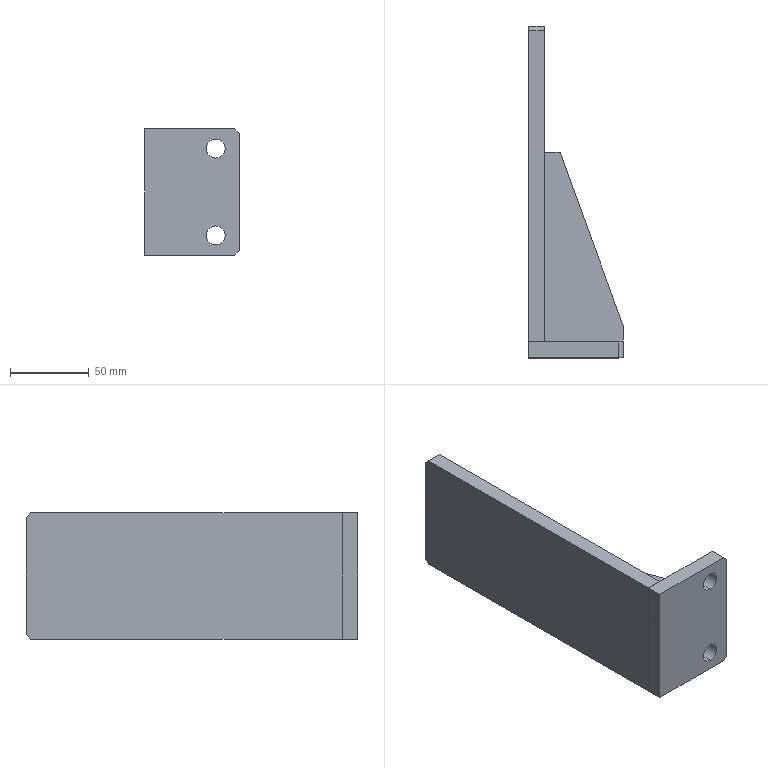Part | SolidWorks | features ICE 3, Chamfer 2, Extrusion 1 | 3 solids | 27 faces | box 60 x 210 x 80 mm | volume 235958 mm3 | plane 23 | cylinder 4 | commonest cylinder face diameters 12 x4
STEP:
#1=CARTESIAN_POINT('',(-30.,202.,40.));
#2=VERTEX_POINT('',#1);
#3=CARTESIAN_POINT('',(-30.,5.,40.));
#4=VERTEX_POINT('',#3);
#5=CARTESIAN_POINT('',(-30.,205.,40.));
#6=DIRECTION('',(0.,-1.,0.));
#7=VECTOR('',#6,1000.);
#8=LINE('',#5,#7);
#9=EDGE_CURVE('',#2,#4,#8,.T.);
#10=ORIENTED_EDGE('',*,*,#9,.F.);
#11=CARTESIAN_POINT('',(-30.,205.,37.));
#12=VERTEX_POINT('',#11);
#13=CARTESIAN_POINT('',(-30.,205.,37.));
#14=DIRECTION('',(0.,0.7071,-0.7071));
#15=VECTOR('',#14,1000.);
#16=LINE('',#13,#15);
#17=EDGE_CURVE('',#2,#12,#16,.T.);
#18=ORIENTED_EDGE('',*,*,#17,.T.);
#19=CARTESIAN_POINT('',(-30.,205.,-37.));
#20=VERTEX_POINT('',#19);
#21=CARTESIAN_POINT('',(-30.,205.,40.));
#22=DIRECTION('',(0.,0.,1.));
#23=VECTOR('',#22,1000.);
#24=LINE('',#21,#23);
#25=EDGE_CURVE('',#20,#12,#24,.T.);
#26=ORIENTED_EDGE('',*,*,#25,.F.);
#27=CARTESIAN_POINT('',(-30.,202.,-40.));
#28=VERTEX_POINT('',#27);
#29=CARTESIAN_POINT('',(-30.,205.,-37.));
#30=DIRECTION('',(0.,-0.7071,-0.7071));
#31=VECTOR('',#30,1000.);
#32=LINE('',#29,#31);
#33=EDGE_CURVE('',#20,#28,#32,.T.);
#34=ORIENTED_EDGE('',*,*,#33,.T.);
#35=CARTESIAN_POINT('',(-30.,5.,-40.));
#36=VERTEX_POINT('',#35);
#37=CARTESIAN_POINT('',(-30.,205.,-40.));
#38=DIRECTION('',(0.,-1.,0.));
#39=VECTOR('',#38,1000.);
#40=LINE('',#37,#39);
#41=EDGE_CURVE('',#28,#36,#40,.T.);
#42=ORIENTED_EDGE('',*,*,#41,.T.);
#43=CARTESIAN_POINT('',(-30.,5.,40.));
#44=DIRECTION('',(0.,0.,1.));
#45=VECTOR('',#44,1000.);
#46=LINE('',#43,#45);
#47=EDGE_CURVE('',#36,#4,#46,.T.);
#48=ORIENTED_EDGE('',*,*,#47,.T.);
#49=EDGE_LOOP('',(#10,#18,#26,#34,#42,#48));
#50=FACE_OUTER_BOUND('',#49,.T.);
#51=CARTESIAN_POINT('',(-30.,205.,40.));
#52=DIRECTION('',(1.,0.,0.));
#53=DIRECTION('',(0.,0.,-1.));
#54=AXIS2_PLACEMENT_3D('',#51,#52,#53);
#55=PLANE('',#54);
#56=ADVANCED_FACE('',(#50),#55,.F.);
#57=CARTESIAN_POINT('',(-20.,202.,40.));
#58=VERTEX_POINT('',#57);
#59=CARTESIAN_POINT('',(-20.,5.,40.));
#60=VERTEX_POINT('',#59);
#61=CARTESIAN_POINT('',(-20.,205.,40.));
#62=DIRECTION('',(0.,-1.,0.));
#63=VECTOR('',#62,1000.);
#64=LINE('',#61,#63);
#65=EDGE_CURVE('',#58,#60,#64,.T.);
#66=ORIENTED_EDGE('',*,*,#65,.F.);
#67=CARTESIAN_POINT('',(-30.,202.,40.));
#68=DIRECTION('',(-1.,0.,0.));
#69=VECTOR('',#68,1000.);
#70=LINE('',#67,#69);
#71=EDGE_CURVE('',#58,#2,#70,.T.);
#72=ORIENTED_EDGE('',*,*,#71,.T.);
#73=ORIENTED_EDGE('',*,*,#9,.T.);
#74=CARTESIAN_POINT('',(-30.,5.,40.));
#75=DIRECTION('',(1.,0.,0.));
#76=VECTOR('',#75,1000.);
#77=LINE('',#74,#76);
#78=EDGE_CURVE('',#4,#60,#77,.T.);
#79=ORIENTED_EDGE('',*,*,#78,.T.);
#80=EDGE_LOOP('',(#66,#72,#73,#79));
#81=FACE_OUTER_BOUND('',#80,.T.);
#82=CARTESIAN_POINT('',(-30.,205.,40.));
#83=DIRECTION('',(0.,0.,-1.));
#84=DIRECTION('',(-1.,0.,0.));
#85=AXIS2_PLACEMENT_3D('',#82,#83,#84);
#86=PLANE('',#85);
#87=ADVANCED_FACE('',(#81),#86,.F.);
#88=CARTESIAN_POINT('',(-20.,205.,37.));
#89=VERTEX_POINT('',#88);
#90=CARTESIAN_POINT('',(-20.,205.,-37.));
#91=VERTEX_POINT('',#90);
#92=CARTESIAN_POINT('',(-20.,205.,40.));
#93=DIRECTION('',(0.,0.,-1.));
#94=VECTOR('',#93,1000.);
#95=LINE('',#92,#94);
#96=EDGE_CURVE('',#89,#91,#95,.T.);
#97=ORIENTED_EDGE('',*,*,#96,.F.);
#98=CARTESIAN_POINT('',(-20.,205.,37.));
#99=DIRECTION('',(0.,-0.7071,0.7071));
#100=VECTOR('',#99,1000.);
#101=LINE('',#98,#100);
#102=EDGE_CURVE('',#89,#58,#101,.T.);
#103=ORIENTED_EDGE('',*,*,#102,.T.);
#104=ORIENTED_EDGE('',*,*,#65,.T.);
#105=CARTESIAN_POINT('',(-20.,5.,-40.));
#106=VERTEX_POINT('',#105);
#107=CARTESIAN_POINT('',(-20.,5.,40.));
#108=DIRECTION('',(0.,0.,-1.));
#109=VECTOR('',#108,1000.);
#110=LINE('',#107,#109);
#111=EDGE_CURVE('',#60,#106,#110,.T.);
#112=ORIENTED_EDGE('',*,*,#111,.T.);
#113=CARTESIAN_POINT('',(-20.,202.,-40.));
#114=VERTEX_POINT('',#113);
#115=CARTESIAN_POINT('',(-20.,205.,-40.));
#116=DIRECTION('',(0.,-1.,0.));
#117=VECTOR('',#116,1000.);
#118=LINE('',#115,#117);
#119=EDGE_CURVE('',#114,#106,#118,.T.);
#120=ORIENTED_EDGE('',*,*,#119,.F.);
#121=CARTESIAN_POINT('',(-20.,205.,-37.));
#122=DIRECTION('',(0.,0.7071,0.7071));
#123=VECTOR('',#122,1000.);
#124=LINE('',#121,#123);
#125=EDGE_CURVE('',#114,#91,#124,.T.);
#126=ORIENTED_EDGE('',*,*,#125,.T.);
#127=EDGE_LOOP('',(#97,#103,#104,#112,#120,#126));
#128=FACE_OUTER_BOUND('',#127,.T.);
#129=CARTESIAN_POINT('',(-20.,205.,40.));
#130=DIRECTION('',(-1.,0.,0.));
#131=DIRECTION('',(0.,0.,1.));
#132=AXIS2_PLACEMENT_3D('',#129,#130,#131);
#133=PLANE('',#132);
#134=ADVANCED_FACE('',(#128),#133,.F.);
#135=ORIENTED_EDGE('',*,*,#41,.F.);
#136=CARTESIAN_POINT('',(-30.,202.,-40.));
#137=DIRECTION('',(1.,0.,0.));
#138=VECTOR('',#137,1000.);
#139=LINE('',#136,#138);
#140=EDGE_CURVE('',#28,#114,#139,.T.);
#141=ORIENTED_EDGE('',*,*,#140,.T.);
#142=ORIENTED_EDGE('',*,*,#119,.T.);
#143=CARTESIAN_POINT('',(-30.,5.,-40.));
#144=DIRECTION('',(-1.,0.,0.));
#145=VECTOR('',#144,1000.);
#146=LINE('',#143,#145);
#147=EDGE_CURVE('',#106,#36,#146,.T.);
#148=ORIENTED_EDGE('',*,*,#147,.T.);
#149=EDGE_LOOP('',(#135,#141,#142,#148));
#150=FACE_OUTER_BOUND('',#149,.T.);
#151=CARTESIAN_POINT('',(-30.,205.,-40.));
#152=DIRECTION('',(0.,0.,1.));
#153=DIRECTION('',(1.,0.,0.));
#154=AXIS2_PLACEMENT_3D('',#151,#152,#153);
#155=PLANE('',#154);
#156=ADVANCED_FACE('',(#150),#155,.F.);
#157=ORIENTED_EDGE('',*,*,#25,.T.);
#158=CARTESIAN_POINT('',(0.,205.,37.));
#159=DIRECTION('',(1.,0.,0.));
#160=VECTOR('',#159,1000.);
#161=LINE('',#158,#160);
#162=EDGE_CURVE('',#12,#89,#161,.T.);
#163=ORIENTED_EDGE('',*,*,#162,.T.);
#164=ORIENTED_EDGE('',*,*,#96,.T.);
#165=CARTESIAN_POINT('',(0.,205.,-37.));
#166=DIRECTION('',(-1.,0.,0.));
#167=VECTOR('',#166,1000.);
#168=LINE('',#165,#167);
#169=EDGE_CURVE('',#91,#20,#168,.T.);
#170=ORIENTED_EDGE('',*,*,#169,.T.);
#171=EDGE_LOOP('',(#157,#163,#164,#170));
#172=FACE_OUTER_BOUND('',#171,.T.);
#173=CARTESIAN_POINT('',(0.,205.,0.));
#174=DIRECTION('',(0.,-1.,0.));
#175=DIRECTION('',(0.,0.,-1.));
#176=AXIS2_PLACEMENT_3D('',#173,#174,#175);
#177=PLANE('',#176);
#178=ADVANCED_FACE('',(#172),#177,.F.);
#179=ORIENTED_EDGE('',*,*,#47,.F.);
#180=ORIENTED_EDGE('',*,*,#147,.F.);
#181=ORIENTED_EDGE('',*,*,#111,.F.);
#182=ORIENTED_EDGE('',*,*,#78,.F.);
#183=EDGE_LOOP('',(#179,#180,#181,#182));
#184=FACE_OUTER_BOUND('',#183,.T.);
#185=CARTESIAN_POINT('',(0.,5.,0.));
#186=DIRECTION('',(0.,-1.,0.));
#187=DIRECTION('',(0.,0.,-1.));
#188=AXIS2_PLACEMENT_3D('',#185,#186,#187);
#189=PLANE('',#188);
#190=ADVANCED_FACE('',(#184),#189,.T.);
#191=ORIENTED_EDGE('',*,*,#17,.F.);
#192=ORIENTED_EDGE('',*,*,#71,.F.);
#193=ORIENTED_EDGE('',*,*,#102,.F.);
#194=ORIENTED_EDGE('',*,*,#162,.F.);
#195=EDGE_LOOP('',(#191,#192,#193,#194));
#196=FACE_OUTER_BOUND('',#195,.T.);
#197=CARTESIAN_POINT('',(0.,205.,37.));
#198=DIRECTION('',(0.,-0.7071,-0.7071));
#199=DIRECTION('',(1.,0.,0.));
#200=AXIS2_PLACEMENT_3D('',#197,#198,#199);
#201=PLANE('',#200);
#202=ADVANCED_FACE('',(#196),#201,.F.);
#203=ORIENTED_EDGE('',*,*,#125,.F.);
#204=ORIENTED_EDGE('',*,*,#140,.F.);
#205=ORIENTED_EDGE('',*,*,#33,.F.);
#206=ORIENTED_EDGE('',*,*,#169,.F.);
#207=EDGE_LOOP('',(#203,#204,#205,#206));
#208=FACE_OUTER_BOUND('',#207,.T.);
#209=CARTESIAN_POINT('',(0.,205.,-37.));
#210=DIRECTION('',(0.,-0.7071,0.7071));
#211=DIRECTION('',(-1.,0.,0.));
#212=AXIS2_PLACEMENT_3D('',#209,#210,#211);
#213=PLANE('',#212);
#214=ADVANCED_FACE('',(#208),#213,.F.);
#215=CLOSED_SHELL('',(#56,#87,#134,#156,#178,#190,#202,#214));
#216=MANIFOLD_SOLID_BREP('',#215);
#217=CARTESIAN_POINT('',(-20.,125.,-4.));
#218=VERTEX_POINT('',#217);
#219=CARTESIAN_POINT('',(-20.,5.,-4.));
#220=VERTEX_POINT('',#219);
#221=CARTESIAN_POINT('',(-20.,5.,-4.));
#222=DIRECTION('',(0.,-1.,0.));
#223=VECTOR('',#222,1000.);
#224=LINE('',#221,#223);
#225=EDGE_CURVE('',#218,#220,#224,.T.);
#226=ORIENTED_EDGE('',*,*,#225,.T.);
#227=CARTESIAN_POINT('',(-20.,5.,4.));
#228=VERTEX_POINT('',#227);
#229=CARTESIAN_POINT('',(-20.,5.,4.));
#230=DIRECTION('',(0.,0.,-1.));
#231=VECTOR('',#230,1000.);
#232=LINE('',#229,#231);
#233=EDGE_CURVE('',#228,#220,#232,.T.);
#234=ORIENTED_EDGE('',*,*,#233,.F.);
#235=CARTESIAN_POINT('',(-20.,125.,4.));
#236=VERTEX_POINT('',#235);
#237=CARTESIAN_POINT('',(-20.,5.,4.));
#238=DIRECTION('',(0.,-1.,0.));
#239=VECTOR('',#238,1000.);
#240=LINE('',#237,#239);
#241=EDGE_CURVE('',#236,#228,#240,.T.);
#242=ORIENTED_EDGE('',*,*,#241,.F.);
#243=CARTESIAN_POINT('',(-20.,125.,4.));
#244=DIRECTION('',(0.,0.,-1.));
#245=VECTOR('',#244,1000.);
#246=LINE('',#243,#245);
#247=EDGE_CURVE('',#236,#218,#246,.T.);
#248=ORIENTED_EDGE('',*,*,#247,.T.);
#249=EDGE_LOOP('',(#226,#234,#242,#248));
#250=FACE_OUTER_BOUND('',#249,.T.);
#251=CARTESIAN_POINT('',(-20.,5.,4.));
#252=DIRECTION('',(1.,0.,0.));
#253=DIRECTION('',(0.,0.,-1.));
#254=AXIS2_PLACEMENT_3D('',#251,#252,#253);
#255=PLANE('',#254);
#256=ADVANCED_FACE('',(#250),#255,.F.);
#257=CARTESIAN_POINT('',(30.,5.,-4.));
#258=VERTEX_POINT('',#257);
#259=CARTESIAN_POINT('',(30.,5.,-4.));
#260=DIRECTION('',(1.,0.,0.));
#261=VECTOR('',#260,1000.);
#262=LINE('',#259,#261);
#263=EDGE_CURVE('',#220,#258,#262,.T.);
#264=ORIENTED_EDGE('',*,*,#263,.T.);
#265=CARTESIAN_POINT('',(30.,5.,4.));
#266=VERTEX_POINT('',#265);
#267=CARTESIAN_POINT('',(30.,5.,4.));
#268=DIRECTION('',(0.,0.,-1.));
#269=VECTOR('',#268,1000.);
#270=LINE('',#267,#269);
#271=EDGE_CURVE('',#266,#258,#270,.T.);
#272=ORIENTED_EDGE('',*,*,#271,.F.);
#273=CARTESIAN_POINT('',(30.,5.,4.));
#274=DIRECTION('',(1.,0.,0.));
#275=VECTOR('',#274,1000.);
#276=LINE('',#273,#275);
#277=EDGE_CURVE('',#228,#266,#276,.T.);
#278=ORIENTED_EDGE('',*,*,#277,.F.);
#279=ORIENTED_EDGE('',*,*,#233,.T.);
#280=EDGE_LOOP('',(#264,#272,#278,#279));
#281=FACE_OUTER_BOUND('',#280,.T.);
#282=CARTESIAN_POINT('',(30.,5.,4.));
#283=DIRECTION('',(0.,1.,0.));
#284=DIRECTION('',(0.,0.,1.));
#285=AXIS2_PLACEMENT_3D('',#282,#283,#284);
#286=PLANE('',#285);
#287=ADVANCED_FACE('',(#281),#286,.F.);
#288=CARTESIAN_POINT('',(30.,15.,-4.));
#289=VERTEX_POINT('',#288);
#290=CARTESIAN_POINT('',(30.,15.,-4.));
#291=DIRECTION('',(0.,1.,0.));
#292=VECTOR('',#291,1000.);
#293=LINE('',#290,#292);
#294=EDGE_CURVE('',#258,#289,#293,.T.);
#295=ORIENTED_EDGE('',*,*,#294,.T.);
#296=CARTESIAN_POINT('',(30.,15.,4.));
#297=VERTEX_POINT('',#296);
#298=CARTESIAN_POINT('',(30.,15.,4.));
#299=DIRECTION('',(0.,0.,-1.));
#300=VECTOR('',#299,1000.);
#301=LINE('',#298,#300);
#302=EDGE_CURVE('',#297,#289,#301,.T.);
#303=ORIENTED_EDGE('',*,*,#302,.F.);
#304=CARTESIAN_POINT('',(30.,15.,4.));
#305=DIRECTION('',(0.,1.,0.));
#306=VECTOR('',#305,1000.);
#307=LINE('',#304,#306);
#308=EDGE_CURVE('',#266,#297,#307,.T.);
#309=ORIENTED_EDGE('',*,*,#308,.F.);
#310=ORIENTED_EDGE('',*,*,#271,.T.);
#311=EDGE_LOOP('',(#295,#303,#309,#310));
#312=FACE_OUTER_BOUND('',#311,.T.);
#313=CARTESIAN_POINT('',(30.,15.,4.));
#314=DIRECTION('',(-1.,0.,0.));
#315=DIRECTION('',(0.,0.,1.));
#316=AXIS2_PLACEMENT_3D('',#313,#314,#315);
#317=PLANE('',#316);
#318=ADVANCED_FACE('',(#312),#317,.F.);
#319=CARTESIAN_POINT('',(-10.,125.,-4.));
#320=VERTEX_POINT('',#319);
#321=CARTESIAN_POINT('',(-10.,125.,-4.));
#322=DIRECTION('',(-0.3417,0.9398,0.));
#323=VECTOR('',#322,1000.);
#324=LINE('',#321,#323);
#325=EDGE_CURVE('',#289,#320,#324,.T.);
#326=ORIENTED_EDGE('',*,*,#325,.T.);
#327=CARTESIAN_POINT('',(-10.,125.,4.));
#328=VERTEX_POINT('',#327);
#329=CARTESIAN_POINT('',(-10.,125.,4.));
#330=DIRECTION('',(0.,0.,-1.));
#331=VECTOR('',#330,1000.);
#332=LINE('',#329,#331);
#333=EDGE_CURVE('',#328,#320,#332,.T.);
#334=ORIENTED_EDGE('',*,*,#333,.F.);
#335=CARTESIAN_POINT('',(-10.,125.,4.));
#336=DIRECTION('',(-0.3417,0.9398,0.));
#337=VECTOR('',#336,1000.);
#338=LINE('',#335,#337);
#339=EDGE_CURVE('',#297,#328,#338,.T.);
#340=ORIENTED_EDGE('',*,*,#339,.F.);
#341=ORIENTED_EDGE('',*,*,#302,.T.);
#342=EDGE_LOOP('',(#326,#334,#340,#341));
#343=FACE_OUTER_BOUND('',#342,.T.);
#344=CARTESIAN_POINT('',(-10.,125.,4.));
#345=DIRECTION('',(-0.9398,-0.3417,0.));
#346=DIRECTION('',(0.3417,-0.9398,0.));
#347=AXIS2_PLACEMENT_3D('',#344,#345,#346);
#348=PLANE('',#347);
#349=ADVANCED_FACE('',(#343),#348,.F.);
#350=CARTESIAN_POINT('',(-20.,125.,-4.));
#351=DIRECTION('',(-1.,0.,0.));
#352=VECTOR('',#351,1000.);
#353=LINE('',#350,#352);
#354=EDGE_CURVE('',#320,#218,#353,.T.);
#355=ORIENTED_EDGE('',*,*,#354,.T.);
#356=ORIENTED_EDGE('',*,*,#247,.F.);
#357=CARTESIAN_POINT('',(-20.,125.,4.));
#358=DIRECTION('',(-1.,0.,0.));
#359=VECTOR('',#358,1000.);
#360=LINE('',#357,#359);
#361=EDGE_CURVE('',#328,#236,#360,.T.);
#362=ORIENTED_EDGE('',*,*,#361,.F.);
#363=ORIENTED_EDGE('',*,*,#333,.T.);
#364=EDGE_LOOP('',(#355,#356,#362,#363));
#365=FACE_OUTER_BOUND('',#364,.T.);
#366=CARTESIAN_POINT('',(-20.,125.,4.));
#367=DIRECTION('',(0.,-1.,0.));
#368=DIRECTION('',(0.,0.,-1.));
#369=AXIS2_PLACEMENT_3D('',#366,#367,#368);
#370=PLANE('',#369);
#371=ADVANCED_FACE('',(#365),#370,.F.);
#372=ORIENTED_EDGE('',*,*,#241,.T.);
#373=ORIENTED_EDGE('',*,*,#277,.T.);
#374=ORIENTED_EDGE('',*,*,#308,.T.);
#375=ORIENTED_EDGE('',*,*,#339,.T.);
#376=ORIENTED_EDGE('',*,*,#361,.T.);
#377=EDGE_LOOP('',(#372,#373,#374,#375,#376));
#378=FACE_OUTER_BOUND('',#377,.T.);
#379=CARTESIAN_POINT('',(0.,0.,4.));
#380=DIRECTION('',(0.,0.,-1.));
#381=DIRECTION('',(-1.,0.,0.));
#382=AXIS2_PLACEMENT_3D('',#379,#380,#381);
#383=PLANE('',#382);
#384=ADVANCED_FACE('',(#378),#383,.F.);
#385=ORIENTED_EDGE('',*,*,#225,.F.);
#386=ORIENTED_EDGE('',*,*,#354,.F.);
#387=ORIENTED_EDGE('',*,*,#325,.F.);
#388=ORIENTED_EDGE('',*,*,#294,.F.);
#389=ORIENTED_EDGE('',*,*,#263,.F.);
#390=EDGE_LOOP('',(#385,#386,#387,#388,#389));
#391=FACE_OUTER_BOUND('',#390,.T.);
#392=CARTESIAN_POINT('',(0.,0.,-4.));
#393=DIRECTION('',(0.,0.,-1.));
#394=DIRECTION('',(-1.,0.,0.));
#395=AXIS2_PLACEMENT_3D('',#392,#393,#394);
#396=PLANE('',#395);
#397=ADVANCED_FACE('',(#391),#396,.T.);
#398=CLOSED_SHELL('',(#256,#287,#318,#349,#371,#384,#397));
#399=MANIFOLD_SOLID_BREP('',#398);
#400=CARTESIAN_POINT('',(15.,-5.,21.5));
#401=VERTEX_POINT('',#400);
#402=CARTESIAN_POINT('',(15.,-5.,33.5));
#403=VERTEX_POINT('',#402);
#404=CARTESIAN_POINT('',(15.,-5.,27.5));
#405=DIRECTION('',(0.,1.,0.));
#406=DIRECTION('',(0.,0.,1.));
#407=AXIS2_PLACEMENT_3D('',#404,#405,#406);
#408=CIRCLE('',#407,6.);
#409=EDGE_CURVE('',#401,#403,#408,.T.);
#410=ORIENTED_EDGE('',*,*,#409,.F.);
#411=CARTESIAN_POINT('',(15.,5.,21.5));
#412=VERTEX_POINT('',#411);
#413=CARTESIAN_POINT('',(15.,-5.,21.5));
#414=DIRECTION('',(0.,1.,0.));
#415=VECTOR('',#414,1000.);
#416=LINE('',#413,#415);
#417=EDGE_CURVE('',#401,#412,#416,.T.);
#418=ORIENTED_EDGE('',*,*,#417,.T.);
#419=CARTESIAN_POINT('',(15.,5.,33.5));
#420=VERTEX_POINT('',#419);
#421=CARTESIAN_POINT('',(15.,5.,27.5));
#422=DIRECTION('',(0.,1.,0.));
#423=DIRECTION('',(0.,0.,1.));
#424=AXIS2_PLACEMENT_3D('',#421,#422,#423);
#425=CIRCLE('',#424,6.);
#426=EDGE_CURVE('',#412,#420,#425,.T.);
#427=ORIENTED_EDGE('',*,*,#426,.T.);
#428=CARTESIAN_POINT('',(15.,-5.,33.5));
#429=DIRECTION('',(0.,1.,0.));
#430=VECTOR('',#429,1000.);
#431=LINE('',#428,#430);
#432=EDGE_CURVE('',#403,#420,#431,.T.);
#433=ORIENTED_EDGE('',*,*,#432,.F.);
#434=EDGE_LOOP('',(#410,#418,#427,#433));
#435=FACE_OUTER_BOUND('',#434,.T.);
#436=CARTESIAN_POINT('',(15.,-5.,27.5));
#437=DIRECTION('',(0.,1.,0.));
#438=DIRECTION('',(0.,0.,1.));
#439=AXIS2_PLACEMENT_3D('',#436,#437,#438);
#440=CYLINDRICAL_SURFACE('',#439,6.);
#441=ADVANCED_FACE('',(#435),#440,.F.);
#442=CARTESIAN_POINT('',(15.,-5.,-33.5));
#443=VERTEX_POINT('',#442);
#444=CARTESIAN_POINT('',(15.,-5.,-21.5));
#445=VERTEX_POINT('',#444);
#446=CARTESIAN_POINT('',(15.,-5.,-27.5));
#447=DIRECTION('',(0.,1.,0.));
#448=DIRECTION('',(0.,0.,-1.));
#449=AXIS2_PLACEMENT_3D('',#446,#447,#448);
#450=CIRCLE('',#449,6.);
#451=EDGE_CURVE('',#443,#445,#450,.T.);
#452=ORIENTED_EDGE('',*,*,#451,.F.);
#453=CARTESIAN_POINT('',(15.,5.,-33.5));
#454=VERTEX_POINT('',#453);
#455=CARTESIAN_POINT('',(15.,-5.,-33.5));
#456=DIRECTION('',(0.,1.,0.));
#457=VECTOR('',#456,1000.);
#458=LINE('',#455,#457);
#459=EDGE_CURVE('',#443,#454,#458,.T.);
#460=ORIENTED_EDGE('',*,*,#459,.T.);
#461=CARTESIAN_POINT('',(15.,5.,-21.5));
#462=VERTEX_POINT('',#461);
#463=CARTESIAN_POINT('',(15.,5.,-27.5));
#464=DIRECTION('',(0.,1.,0.));
#465=DIRECTION('',(0.,0.,-1.));
#466=AXIS2_PLACEMENT_3D('',#463,#464,#465);
#467=CIRCLE('',#466,6.);
#468=EDGE_CURVE('',#454,#462,#467,.T.);
#469=ORIENTED_EDGE('',*,*,#468,.T.);
#470=CARTESIAN_POINT('',(15.,-5.,-21.5));
#471=DIRECTION('',(0.,1.,0.));
#472=VECTOR('',#471,1000.);
#473=LINE('',#470,#472);
#474=EDGE_CURVE('',#445,#462,#473,.T.);
#475=ORIENTED_EDGE('',*,*,#474,.F.);
#476=EDGE_LOOP('',(#452,#460,#469,#475));
#477=FACE_OUTER_BOUND('',#476,.T.);
#478=CARTESIAN_POINT('',(15.,-5.,-27.5));
#479=DIRECTION('',(0.,1.,0.));
#480=DIRECTION('',(0.,0.,1.));
#481=AXIS2_PLACEMENT_3D('',#478,#479,#480);
#482=CYLINDRICAL_SURFACE('',#481,6.);
#483=ADVANCED_FACE('',(#477),#482,.F.);
#484=CARTESIAN_POINT('',(30.,-5.,37.));
#485=VERTEX_POINT('',#484);
#486=CARTESIAN_POINT('',(30.,-5.,-37.));
#487=VERTEX_POINT('',#486);
#488=CARTESIAN_POINT('',(30.,-5.,40.));
#489=DIRECTION('',(0.,0.,-1.));
#490=VECTOR('',#489,1000.);
#491=LINE('',#488,#490);
#492=EDGE_CURVE('',#485,#487,#491,.T.);
#493=ORIENTED_EDGE('',*,*,#492,.T.);
#494=CARTESIAN_POINT('',(30.,5.,-37.));
#495=VERTEX_POINT('',#494);
#496=CARTESIAN_POINT('',(30.,5.,-37.));
#497=DIRECTION('',(0.,1.,0.));
#498=VECTOR('',#497,1000.);
#499=LINE('',#496,#498);
#500=EDGE_CURVE('',#487,#495,#499,.T.);
#501=ORIENTED_EDGE('',*,*,#500,.T.);
#502=CARTESIAN_POINT('',(30.,5.,37.));
#503=VERTEX_POINT('',#502);
#504=CARTESIAN_POINT('',(30.,5.,40.));
#505=DIRECTION('',(0.,0.,-1.));
#506=VECTOR('',#505,1000.);
#507=LINE('',#504,#506);
#508=EDGE_CURVE('',#503,#495,#507,.T.);
#509=ORIENTED_EDGE('',*,*,#508,.F.);
#510=CARTESIAN_POINT('',(30.,5.,37.));
#511=DIRECTION('',(0.,-1.,0.));
#512=VECTOR('',#511,1000.);
#513=LINE('',#510,#512);
#514=EDGE_CURVE('',#503,#485,#513,.T.);
#515=ORIENTED_EDGE('',*,*,#514,.T.);
#516=EDGE_LOOP('',(#493,#501,#509,#515));
#517=FACE_OUTER_BOUND('',#516,.T.);
#518=CARTESIAN_POINT('',(30.,5.,40.));
#519=DIRECTION('',(-1.,0.,0.));
#520=DIRECTION('',(0.,0.,1.));
#521=AXIS2_PLACEMENT_3D('',#518,#519,#520);
#522=PLANE('',#521);
#523=ADVANCED_FACE('',(#517),#522,.F.);
#524=CARTESIAN_POINT('',(27.,5.,-40.));
#525=VERTEX_POINT('',#524);
#526=CARTESIAN_POINT('',(-30.,5.,-40.));
#527=VERTEX_POINT('',#526);
#528=CARTESIAN_POINT('',(-30.,5.,-40.));
#529=DIRECTION('',(-1.,0.,0.));
#530=VECTOR('',#529,1000.);
#531=LINE('',#528,#530);
#532=EDGE_CURVE('',#525,#527,#531,.T.);
#533=ORIENTED_EDGE('',*,*,#532,.F.);
#534=CARTESIAN_POINT('',(27.,-5.,-40.));
#535=VERTEX_POINT('',#534);
#536=CARTESIAN_POINT('',(27.,5.,-40.));
#537=DIRECTION('',(0.,-1.,0.));
#538=VECTOR('',#537,1000.);
#539=LINE('',#536,#538);
#540=EDGE_CURVE('',#525,#535,#539,.T.);
#541=ORIENTED_EDGE('',*,*,#540,.T.);
#542=CARTESIAN_POINT('',(-30.,-5.,-40.));
#543=VERTEX_POINT('',#542);
#544=CARTESIAN_POINT('',(-30.,-5.,-40.));
#545=DIRECTION('',(-1.,0.,0.));
#546=VECTOR('',#545,1000.);
#547=LINE('',#544,#546);
#548=EDGE_CURVE('',#535,#543,#547,.T.);
#549=ORIENTED_EDGE('',*,*,#548,.T.);
#550=CARTESIAN_POINT('',(-30.,5.,-40.));
#551=DIRECTION('',(0.,-1.,0.));
#552=VECTOR('',#551,1000.);
#553=LINE('',#550,#552);
#554=EDGE_CURVE('',#527,#543,#553,.T.);
#555=ORIENTED_EDGE('',*,*,#554,.F.);
#556=EDGE_LOOP('',(#533,#541,#549,#555));
#557=FACE_OUTER_BOUND('',#556,.T.);
#558=CARTESIAN_POINT('',(-30.,5.,-40.));
#559=DIRECTION('',(0.,0.,1.));
#560=DIRECTION('',(1.,0.,0.));
#561=AXIS2_PLACEMENT_3D('',#558,#559,#560);
#562=PLANE('',#561);
#563=ADVANCED_FACE('',(#557),#562,.F.);
#564=CARTESIAN_POINT('',(-30.,-5.,40.));
#565=VERTEX_POINT('',#564);
#566=CARTESIAN_POINT('',(-30.,-5.,40.));
#567=DIRECTION('',(0.,0.,1.));
#568=VECTOR('',#567,1000.);
#569=LINE('',#566,#568);
#570=EDGE_CURVE('',#543,#565,#569,.T.);
#571=ORIENTED_EDGE('',*,*,#570,.T.);
#572=CARTESIAN_POINT('',(-30.,5.,40.));
#573=VERTEX_POINT('',#572);
#574=CARTESIAN_POINT('',(-30.,5.,40.));
#575=DIRECTION('',(0.,-1.,0.));
#576=VECTOR('',#575,1000.);
#577=LINE('',#574,#576);
#578=EDGE_CURVE('',#573,#565,#577,.T.);
#579=ORIENTED_EDGE('',*,*,#578,.F.);
#580=CARTESIAN_POINT('',(-30.,5.,40.));
#581=DIRECTION('',(0.,0.,1.));
#582=VECTOR('',#581,1000.);
#583=LINE('',#580,#582);
#584=EDGE_CURVE('',#527,#573,#583,.T.);
#585=ORIENTED_EDGE('',*,*,#584,.F.);
#586=ORIENTED_EDGE('',*,*,#554,.T.);
#587=EDGE_LOOP('',(#571,#579,#585,#586));
#588=FACE_OUTER_BOUND('',#587,.T.);
#589=CARTESIAN_POINT('',(-30.,5.,40.));
#590=DIRECTION('',(1.,0.,0.));
#591=DIRECTION('',(0.,0.,-1.));
#592=AXIS2_PLACEMENT_3D('',#589,#590,#591);
#593=PLANE('',#592);
#594=ADVANCED_FACE('',(#588),#593,.F.);
#595=CARTESIAN_POINT('',(27.,-5.,40.));
#596=VERTEX_POINT('',#595);
#597=CARTESIAN_POINT('',(-30.,-5.,40.));
#598=DIRECTION('',(1.,0.,0.));
#599=VECTOR('',#598,1000.);
#600=LINE('',#597,#599);
#601=EDGE_CURVE('',#565,#596,#600,.T.);
#602=ORIENTED_EDGE('',*,*,#601,.T.);
#603=CARTESIAN_POINT('',(27.,5.,40.));
#604=VERTEX_POINT('',#603);
#605=CARTESIAN_POINT('',(27.,5.,40.));
#606=DIRECTION('',(0.,1.,0.));
#607=VECTOR('',#606,1000.);
#608=LINE('',#605,#607);
#609=EDGE_CURVE('',#596,#604,#608,.T.);
#610=ORIENTED_EDGE('',*,*,#609,.T.);
#611=CARTESIAN_POINT('',(-30.,5.,40.));
#612=DIRECTION('',(1.,0.,0.));
#613=VECTOR('',#612,1000.);
#614=LINE('',#611,#613);
#615=EDGE_CURVE('',#573,#604,#614,.T.);
#616=ORIENTED_EDGE('',*,*,#615,.F.);
#617=ORIENTED_EDGE('',*,*,#578,.T.);
#618=EDGE_LOOP('',(#602,#610,#616,#617));
#619=FACE_OUTER_BOUND('',#618,.T.);
#620=CARTESIAN_POINT('',(-30.,5.,40.));
#621=DIRECTION('',(0.,0.,-1.));
#622=DIRECTION('',(-1.,0.,0.));
#623=AXIS2_PLACEMENT_3D('',#620,#621,#622);
#624=PLANE('',#623);
#625=ADVANCED_FACE('',(#619),#624,.F.);
#626=CARTESIAN_POINT('',(15.,5.,27.5));
#627=DIRECTION('',(0.,1.,0.));
#628=DIRECTION('',(0.,0.,1.));
#629=AXIS2_PLACEMENT_3D('',#626,#627,#628);
#630=CIRCLE('',#629,6.);
#631=EDGE_CURVE('',#420,#412,#630,.T.);
#632=ORIENTED_EDGE('',*,*,#631,.F.);
#633=ORIENTED_EDGE('',*,*,#426,.F.);
#634=EDGE_LOOP('',(#632,#633));
#635=FACE_BOUND('',#634,.T.);
#636=CARTESIAN_POINT('',(15.,5.,-27.5));
#637=DIRECTION('',(0.,1.,0.));
#638=DIRECTION('',(0.,0.,-1.));
#639=AXIS2_PLACEMENT_3D('',#636,#637,#638);
#640=CIRCLE('',#639,6.);
#641=EDGE_CURVE('',#462,#454,#640,.T.);
#642=ORIENTED_EDGE('',*,*,#641,.F.);
#643=ORIENTED_EDGE('',*,*,#468,.F.);
#644=EDGE_LOOP('',(#642,#643));
#645=FACE_BOUND('',#644,.T.);
#646=ORIENTED_EDGE('',*,*,#508,.T.);
#647=CARTESIAN_POINT('',(27.,5.,-40.));
#648=DIRECTION('',(-0.7071,0.,-0.7071));
#649=VECTOR('',#648,1000.);
#650=LINE('',#647,#649);
#651=EDGE_CURVE('',#495,#525,#650,.T.);
#652=ORIENTED_EDGE('',*,*,#651,.T.);
#653=ORIENTED_EDGE('',*,*,#532,.T.);
#654=ORIENTED_EDGE('',*,*,#584,.T.);
#655=ORIENTED_EDGE('',*,*,#615,.T.);
#656=CARTESIAN_POINT('',(30.,5.,37.));
#657=DIRECTION('',(0.7071,0.,-0.7071));
#658=VECTOR('',#657,1000.);
#659=LINE('',#656,#658);
#660=EDGE_CURVE('',#604,#503,#659,.T.);
#661=ORIENTED_EDGE('',*,*,#660,.T.);
#662=EDGE_LOOP('',(#646,#652,#653,#654,#655,#661));
#663=FACE_OUTER_BOUND('',#662,.T.);
#664=CARTESIAN_POINT('',(0.,5.,0.));
#665=DIRECTION('',(0.,-1.,0.));
#666=DIRECTION('',(0.,0.,-1.));
#667=AXIS2_PLACEMENT_3D('',#664,#665,#666);
#668=PLANE('',#667);
#669=ADVANCED_FACE('',(#635,#645,#663),#668,.F.);
#670=CARTESIAN_POINT('',(15.,-5.,27.5));
#671=DIRECTION('',(0.,1.,0.));
#672=DIRECTION('',(0.,0.,1.));
#673=AXIS2_PLACEMENT_3D('',#670,#671,#672);
#674=CIRCLE('',#673,6.);
#675=EDGE_CURVE('',#403,#401,#674,.T.);
#676=ORIENTED_EDGE('',*,*,#675,.T.);
#677=ORIENTED_EDGE('',*,*,#409,.T.);
#678=EDGE_LOOP('',(#676,#677));
#679=FACE_BOUND('',#678,.T.);
#680=CARTESIAN_POINT('',(15.,-5.,-27.5));
#681=DIRECTION('',(0.,1.,0.));
#682=DIRECTION('',(0.,0.,-1.));
#683=AXIS2_PLACEMENT_3D('',#680,#681,#682);
#684=CIRCLE('',#683,6.);
#685=EDGE_CURVE('',#445,#443,#684,.T.);
#686=ORIENTED_EDGE('',*,*,#685,.T.);
#687=ORIENTED_EDGE('',*,*,#451,.T.);
#688=EDGE_LOOP('',(#686,#687));
#689=FACE_BOUND('',#688,.T.);
#690=ORIENTED_EDGE('',*,*,#548,.F.);
#691=CARTESIAN_POINT('',(33.5,-5.,-33.5));
#692=DIRECTION('',(0.7071,0.,0.7071));
#693=VECTOR('',#692,1000.);
#694=LINE('',#691,#693);
#695=EDGE_CURVE('',#535,#487,#694,.T.);
#696=ORIENTED_EDGE('',*,*,#695,.T.);
#697=ORIENTED_EDGE('',*,*,#492,.F.);
#698=CARTESIAN_POINT('',(33.5,-5.,33.5));
#699=DIRECTION('',(-0.7071,0.,0.7071));
#700=VECTOR('',#699,1000.);
#701=LINE('',#698,#700);
#702=EDGE_CURVE('',#485,#596,#701,.T.);
#703=ORIENTED_EDGE('',*,*,#702,.T.);
#704=ORIENTED_EDGE('',*,*,#601,.F.);
#705=ORIENTED_EDGE('',*,*,#570,.F.);
#706=EDGE_LOOP('',(#690,#696,#697,#703,#704,#705));
#707=FACE_OUTER_BOUND('',#706,.T.);
#708=CARTESIAN_POINT('',(0.,-5.,0.));
#709=DIRECTION('',(0.,-1.,0.));
#710=DIRECTION('',(0.,0.,-1.));
#711=AXIS2_PLACEMENT_3D('',#708,#709,#710);
#712=PLANE('',#711);
#713=ADVANCED_FACE('',(#679,#689,#707),#712,.T.);
#714=ORIENTED_EDGE('',*,*,#651,.F.);
#715=ORIENTED_EDGE('',*,*,#500,.F.);
#716=ORIENTED_EDGE('',*,*,#695,.F.);
#717=ORIENTED_EDGE('',*,*,#540,.F.);
#718=EDGE_LOOP('',(#714,#715,#716,#717));
#719=FACE_OUTER_BOUND('',#718,.T.);
#720=CARTESIAN_POINT('',(27.,5.,-40.));
#721=DIRECTION('',(-0.7071,0.,0.7071));
#722=DIRECTION('',(0.,-1.,0.));
#723=AXIS2_PLACEMENT_3D('',#720,#721,#722);
#724=PLANE('',#723);
#725=ADVANCED_FACE('',(#719),#724,.F.);
#726=ORIENTED_EDGE('',*,*,#660,.F.);
#727=ORIENTED_EDGE('',*,*,#609,.F.);
#728=ORIENTED_EDGE('',*,*,#702,.F.);
#729=ORIENTED_EDGE('',*,*,#514,.F.);
#730=EDGE_LOOP('',(#726,#727,#728,#729));
#731=FACE_OUTER_BOUND('',#730,.T.);
#732=CARTESIAN_POINT('',(30.,5.,37.));
#733=DIRECTION('',(-0.7071,0.,-0.7071));
#734=DIRECTION('',(0.,-1.,0.));
#735=AXIS2_PLACEMENT_3D('',#732,#733,#734);
#736=PLANE('',#735);
#737=ADVANCED_FACE('',(#731),#736,.F.);
#738=ORIENTED_EDGE('',*,*,#459,.F.);
#739=ORIENTED_EDGE('',*,*,#685,.F.);
#740=ORIENTED_EDGE('',*,*,#474,.T.);
#741=ORIENTED_EDGE('',*,*,#641,.T.);
#742=EDGE_LOOP('',(#738,#739,#740,#741));
#743=FACE_OUTER_BOUND('',#742,.T.);
#744=CARTESIAN_POINT('',(15.,-5.,-27.5));
#745=DIRECTION('',(0.,1.,0.));
#746=DIRECTION('',(0.,0.,1.));
#747=AXIS2_PLACEMENT_3D('',#744,#745,#746);
#748=CYLINDRICAL_SURFACE('',#747,6.);
#749=ADVANCED_FACE('',(#743),#748,.F.);
#750=ORIENTED_EDGE('',*,*,#417,.F.);
#751=ORIENTED_EDGE('',*,*,#675,.F.);
#752=ORIENTED_EDGE('',*,*,#432,.T.);
#753=ORIENTED_EDGE('',*,*,#631,.T.);
#754=EDGE_LOOP('',(#750,#751,#752,#753));
#755=FACE_OUTER_BOUND('',#754,.T.);
#756=CARTESIAN_POINT('',(15.,-5.,27.5));
#757=DIRECTION('',(0.,1.,0.));
#758=DIRECTION('',(0.,0.,1.));
#759=AXIS2_PLACEMENT_3D('',#756,#757,#758);
#760=CYLINDRICAL_SURFACE('',#759,6.);
#761=ADVANCED_FACE('',(#755),#760,.F.);
#762=CLOSED_SHELL('',(#441,#483,#523,#563,#594,#625,#669,#713,#725,#737,#749,#761));
#763=MANIFOLD_SOLID_BREP('',#762);
#764=CARTESIAN_POINT('',(0.,0.,0.));
#765=DIRECTION('',(0.,0.,1.));
#766=DIRECTION('',(1.,0.,0.));
#767=AXIS2_PLACEMENT_3D('',#764,#765,#766);
#768=(LENGTH_UNIT()NAMED_UNIT(*)SI_UNIT(.MILLI.,.METRE.));
#769=UNCERTAINTY_MEASURE_WITH_UNIT(LENGTH_MEASURE(0.00001),#768,'','');
#770=(NAMED_UNIT(*)PLANE_ANGLE_UNIT()SI_UNIT($,.RADIAN.));
#771=(NAMED_UNIT(*)SI_UNIT($,.STERADIAN.)SOLID_ANGLE_UNIT());
#772=(GEOMETRIC_REPRESENTATION_CONTEXT(3)GLOBAL_UNCERTAINTY_ASSIGNED_CONTEXT((#769))GLOBAL_UNIT_ASSIGNED_CONTEXT((#768,#770,#771))REPRESENTATION_CONTEXT('',''));
#773=ADVANCED_BREP_SHAPE_REPRESENTATION('',(#216,#399,#763,#767),#772);